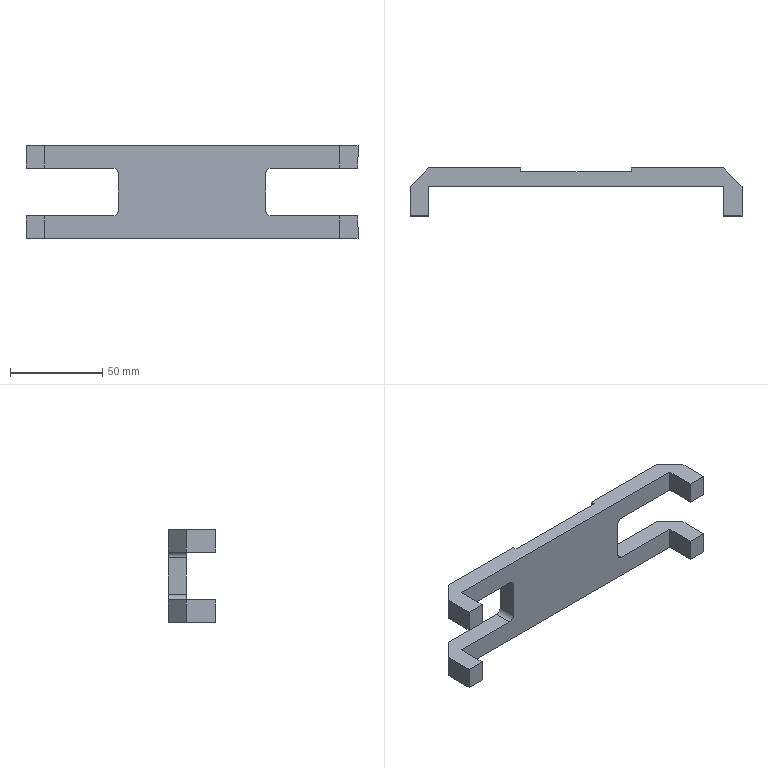Part | SolidWorks | features Cut 2, Chamfer 1, Extrusion 1, Fillet 1, ICE 1, MirrorPattern 1 | 1 solid | 34 faces | box 180 x 26 x 50 mm | volume 63357 mm3 | plane 30 | cylinder 4 | commonest cylinder face diameters 6 x4
STEP:
#1=CARTESIAN_POINT('',(30.,10.,25.));
#2=VERTEX_POINT('',#1);
#3=CARTESIAN_POINT('',(30.,10.,-25.));
#4=VERTEX_POINT('',#3);
#5=CARTESIAN_POINT('',(30.,10.,25.));
#6=DIRECTION('',(0.,0.,-1.));
#7=VECTOR('',#6,1000.);
#8=LINE('',#5,#7);
#9=EDGE_CURVE('',#2,#4,#8,.T.);
#10=ORIENTED_EDGE('',*,*,#9,.F.);
#11=CARTESIAN_POINT('',(80.,10.,25.));
#12=VERTEX_POINT('',#11);
#13=CARTESIAN_POINT('',(-90.,10.,25.));
#14=DIRECTION('',(1.,0.,0.));
#15=VECTOR('',#14,1000.);
#16=LINE('',#13,#15);
#17=EDGE_CURVE('',#2,#12,#16,.T.);
#18=ORIENTED_EDGE('',*,*,#17,.T.);
#19=CARTESIAN_POINT('',(80.,10.,13.));
#20=VERTEX_POINT('',#19);
#21=CARTESIAN_POINT('',(80.,10.,13.));
#22=DIRECTION('',(0.,0.,-1.));
#23=VECTOR('',#22,1000.);
#24=LINE('',#21,#23);
#25=EDGE_CURVE('',#12,#20,#24,.T.);
#26=ORIENTED_EDGE('',*,*,#25,.T.);
#27=CARTESIAN_POINT('',(43.,10.,13.));
#28=VERTEX_POINT('',#27);
#29=CARTESIAN_POINT('',(90.,10.,13.));
#30=DIRECTION('',(-1.,0.,0.));
#31=VECTOR('',#30,1000.);
#32=LINE('',#29,#31);
#33=EDGE_CURVE('',#20,#28,#32,.T.);
#34=ORIENTED_EDGE('',*,*,#33,.T.);
#35=CARTESIAN_POINT('',(40.,10.,10.));
#36=VERTEX_POINT('',#35);
#37=CARTESIAN_POINT('',(43.,10.,10.));
#38=DIRECTION('',(0.,-1.,0.));
#39=DIRECTION('',(0.,0.,1.));
#40=AXIS2_PLACEMENT_3D('',#37,#38,#39);
#41=CIRCLE('',#40,3.);
#42=EDGE_CURVE('',#28,#36,#41,.T.);
#43=ORIENTED_EDGE('',*,*,#42,.T.);
#44=CARTESIAN_POINT('',(40.,10.,-10.));
#45=VERTEX_POINT('',#44);
#46=CARTESIAN_POINT('',(40.,10.,-13.));
#47=DIRECTION('',(0.,0.,-1.));
#48=VECTOR('',#47,1000.);
#49=LINE('',#46,#48);
#50=EDGE_CURVE('',#36,#45,#49,.T.);
#51=ORIENTED_EDGE('',*,*,#50,.T.);
#52=CARTESIAN_POINT('',(43.,10.,-13.));
#53=VERTEX_POINT('',#52);
#54=CARTESIAN_POINT('',(43.,10.,-10.));
#55=DIRECTION('',(0.,-1.,0.));
#56=DIRECTION('',(0.,0.,1.));
#57=AXIS2_PLACEMENT_3D('',#54,#55,#56);
#58=CIRCLE('',#57,3.);
#59=EDGE_CURVE('',#45,#53,#58,.T.);
#60=ORIENTED_EDGE('',*,*,#59,.T.);
#61=CARTESIAN_POINT('',(80.,10.,-13.));
#62=VERTEX_POINT('',#61);
#63=CARTESIAN_POINT('',(90.,10.,-13.));
#64=DIRECTION('',(1.,0.,0.));
#65=VECTOR('',#64,1000.);
#66=LINE('',#63,#65);
#67=EDGE_CURVE('',#53,#62,#66,.T.);
#68=ORIENTED_EDGE('',*,*,#67,.T.);
#69=CARTESIAN_POINT('',(80.,10.,-25.));
#70=VERTEX_POINT('',#69);
#71=CARTESIAN_POINT('',(80.,10.,-25.));
#72=DIRECTION('',(0.,0.,-1.));
#73=VECTOR('',#72,1000.);
#74=LINE('',#71,#73);
#75=EDGE_CURVE('',#62,#70,#74,.T.);
#76=ORIENTED_EDGE('',*,*,#75,.T.);
#77=CARTESIAN_POINT('',(-90.,10.,-25.));
#78=DIRECTION('',(-1.,0.,0.));
#79=VECTOR('',#78,1000.);
#80=LINE('',#77,#79);
#81=EDGE_CURVE('',#70,#4,#80,.T.);
#82=ORIENTED_EDGE('',*,*,#81,.T.);
#83=EDGE_LOOP('',(#10,#18,#26,#34,#43,#51,#60,#68,#76,#82));
#84=FACE_OUTER_BOUND('',#83,.T.);
#85=CARTESIAN_POINT('',(0.,10.,0.));
#86=DIRECTION('',(0.,1.,0.));
#87=DIRECTION('',(0.,0.,1.));
#88=AXIS2_PLACEMENT_3D('',#85,#86,#87);
#89=PLANE('',#88);
#90=ADVANCED_FACE('',(#84),#89,.T.);
#91=CARTESIAN_POINT('',(80.,0.,13.));
#92=VERTEX_POINT('',#91);
#93=CARTESIAN_POINT('',(43.,0.,13.));
#94=VERTEX_POINT('',#93);
#95=CARTESIAN_POINT('',(0.,0.,13.));
#96=DIRECTION('',(-1.,0.,0.));
#97=VECTOR('',#96,1000.);
#98=LINE('',#95,#97);
#99=EDGE_CURVE('',#92,#94,#98,.T.);
#100=ORIENTED_EDGE('',*,*,#99,.F.);
#101=CARTESIAN_POINT('',(80.,0.,25.));
#102=VERTEX_POINT('',#101);
#103=CARTESIAN_POINT('',(80.,0.,-25.));
#104=DIRECTION('',(0.,0.,-1.));
#105=VECTOR('',#104,1000.);
#106=LINE('',#103,#105);
#107=EDGE_CURVE('',#102,#92,#106,.T.);
#108=ORIENTED_EDGE('',*,*,#107,.F.);
#109=CARTESIAN_POINT('',(-80.,0.,25.));
#110=VERTEX_POINT('',#109);
#111=CARTESIAN_POINT('',(-90.,0.,25.));
#112=DIRECTION('',(1.,0.,0.));
#113=VECTOR('',#112,1000.);
#114=LINE('',#111,#113);
#115=EDGE_CURVE('',#110,#102,#114,.T.);
#116=ORIENTED_EDGE('',*,*,#115,.F.);
#117=CARTESIAN_POINT('',(-80.,0.,13.));
#118=VERTEX_POINT('',#117);
#119=CARTESIAN_POINT('',(-80.,0.,-25.));
#120=DIRECTION('',(0.,0.,1.));
#121=VECTOR('',#120,1000.);
#122=LINE('',#119,#121);
#123=EDGE_CURVE('',#118,#110,#122,.T.);
#124=ORIENTED_EDGE('',*,*,#123,.F.);
#125=CARTESIAN_POINT('',(-43.,0.,13.));
#126=VERTEX_POINT('',#125);
#127=CARTESIAN_POINT('',(0.,0.,13.));
#128=DIRECTION('',(1.,0.,0.));
#129=VECTOR('',#128,1000.);
#130=LINE('',#127,#129);
#131=EDGE_CURVE('',#118,#126,#130,.T.);
#132=ORIENTED_EDGE('',*,*,#131,.T.);
#133=CARTESIAN_POINT('',(-40.,0.,10.));
#134=VERTEX_POINT('',#133);
#135=CARTESIAN_POINT('',(-43.,0.,10.));
#136=DIRECTION('',(0.,1.,0.));
#137=DIRECTION('',(0.,0.,1.));
#138=AXIS2_PLACEMENT_3D('',#135,#136,#137);
#139=CIRCLE('',#138,3.);
#140=EDGE_CURVE('',#126,#134,#139,.T.);
#141=ORIENTED_EDGE('',*,*,#140,.T.);
#142=CARTESIAN_POINT('',(-40.,0.,-10.));
#143=VERTEX_POINT('',#142);
#144=CARTESIAN_POINT('',(-40.,0.,0.));
#145=DIRECTION('',(0.,0.,-1.));
#146=VECTOR('',#145,1000.);
#147=LINE('',#144,#146);
#148=EDGE_CURVE('',#134,#143,#147,.T.);
#149=ORIENTED_EDGE('',*,*,#148,.T.);
#150=CARTESIAN_POINT('',(-43.,0.,-13.));
#151=VERTEX_POINT('',#150);
#152=CARTESIAN_POINT('',(-43.,0.,-10.));
#153=DIRECTION('',(0.,1.,0.));
#154=DIRECTION('',(0.,0.,1.));
#155=AXIS2_PLACEMENT_3D('',#152,#153,#154);
#156=CIRCLE('',#155,3.);
#157=EDGE_CURVE('',#143,#151,#156,.T.);
#158=ORIENTED_EDGE('',*,*,#157,.T.);
#159=CARTESIAN_POINT('',(-80.,0.,-13.));
#160=VERTEX_POINT('',#159);
#161=CARTESIAN_POINT('',(0.,0.,-13.));
#162=DIRECTION('',(-1.,0.,0.));
#163=VECTOR('',#162,1000.);
#164=LINE('',#161,#163);
#165=EDGE_CURVE('',#151,#160,#164,.T.);
#166=ORIENTED_EDGE('',*,*,#165,.T.);
#167=CARTESIAN_POINT('',(-80.,0.,-25.));
#168=VERTEX_POINT('',#167);
#169=CARTESIAN_POINT('',(-80.,0.,-25.));
#170=DIRECTION('',(0.,0.,1.));
#171=VECTOR('',#170,1000.);
#172=LINE('',#169,#171);
#173=EDGE_CURVE('',#168,#160,#172,.T.);
#174=ORIENTED_EDGE('',*,*,#173,.F.);
#175=CARTESIAN_POINT('',(80.,0.,-25.));
#176=VERTEX_POINT('',#175);
#177=CARTESIAN_POINT('',(-90.,0.,-25.));
#178=DIRECTION('',(-1.,0.,0.));
#179=VECTOR('',#178,1000.);
#180=LINE('',#177,#179);
#181=EDGE_CURVE('',#176,#168,#180,.T.);
#182=ORIENTED_EDGE('',*,*,#181,.F.);
#183=CARTESIAN_POINT('',(80.,0.,-13.));
#184=VERTEX_POINT('',#183);
#185=CARTESIAN_POINT('',(80.,0.,-25.));
#186=DIRECTION('',(0.,0.,-1.));
#187=VECTOR('',#186,1000.);
#188=LINE('',#185,#187);
#189=EDGE_CURVE('',#184,#176,#188,.T.);
#190=ORIENTED_EDGE('',*,*,#189,.F.);
#191=CARTESIAN_POINT('',(43.,0.,-13.));
#192=VERTEX_POINT('',#191);
#193=CARTESIAN_POINT('',(0.,0.,-13.));
#194=DIRECTION('',(1.,0.,0.));
#195=VECTOR('',#194,1000.);
#196=LINE('',#193,#195);
#197=EDGE_CURVE('',#192,#184,#196,.T.);
#198=ORIENTED_EDGE('',*,*,#197,.F.);
#199=CARTESIAN_POINT('',(40.,0.,-10.));
#200=VERTEX_POINT('',#199);
#201=CARTESIAN_POINT('',(43.,0.,-10.));
#202=DIRECTION('',(0.,1.,0.));
#203=DIRECTION('',(0.,0.,1.));
#204=AXIS2_PLACEMENT_3D('',#201,#202,#203);
#205=CIRCLE('',#204,3.);
#206=EDGE_CURVE('',#192,#200,#205,.T.);
#207=ORIENTED_EDGE('',*,*,#206,.T.);
#208=CARTESIAN_POINT('',(40.,0.,10.));
#209=VERTEX_POINT('',#208);
#210=CARTESIAN_POINT('',(40.,0.,0.));
#211=DIRECTION('',(0.,0.,-1.));
#212=VECTOR('',#211,1000.);
#213=LINE('',#210,#212);
#214=EDGE_CURVE('',#209,#200,#213,.T.);
#215=ORIENTED_EDGE('',*,*,#214,.F.);
#216=CARTESIAN_POINT('',(43.,0.,10.));
#217=DIRECTION('',(0.,1.,0.));
#218=DIRECTION('',(0.,0.,1.));
#219=AXIS2_PLACEMENT_3D('',#216,#217,#218);
#220=CIRCLE('',#219,3.);
#221=EDGE_CURVE('',#209,#94,#220,.T.);
#222=ORIENTED_EDGE('',*,*,#221,.T.);
#223=EDGE_LOOP('',(#100,#108,#116,#124,#132,#141,#149,#158,#166,#174,#182,#190,#198,#207,#215,#222));
#224=FACE_OUTER_BOUND('',#223,.T.);
#225=CARTESIAN_POINT('',(0.,0.,0.));
#226=DIRECTION('',(0.,1.,0.));
#227=DIRECTION('',(0.,0.,1.));
#228=AXIS2_PLACEMENT_3D('',#225,#226,#227);
#229=PLANE('',#228);
#230=ADVANCED_FACE('',(#224),#229,.F.);
#231=CARTESIAN_POINT('',(90.,-16.,13.));
#232=VERTEX_POINT('',#231);
#233=CARTESIAN_POINT('',(90.,0.,13.));
#234=VERTEX_POINT('',#233);
#235=CARTESIAN_POINT('',(90.,-16.,13.));
#236=DIRECTION('',(0.,1.,0.));
#237=VECTOR('',#236,1000.);
#238=LINE('',#235,#237);
#239=EDGE_CURVE('',#232,#234,#238,.T.);
#240=ORIENTED_EDGE('',*,*,#239,.T.);
#241=CARTESIAN_POINT('',(90.,0.,25.));
#242=VERTEX_POINT('',#241);
#243=CARTESIAN_POINT('',(90.,0.,25.));
#244=DIRECTION('',(0.,0.,1.));
#245=VECTOR('',#244,1000.);
#246=LINE('',#243,#245);
#247=EDGE_CURVE('',#234,#242,#246,.T.);
#248=ORIENTED_EDGE('',*,*,#247,.T.);
#249=CARTESIAN_POINT('',(90.,-16.,25.));
#250=VERTEX_POINT('',#249);
#251=CARTESIAN_POINT('',(90.,10.,25.));
#252=DIRECTION('',(0.,-1.,0.));
#253=VECTOR('',#252,1000.);
#254=LINE('',#251,#253);
#255=EDGE_CURVE('',#242,#250,#254,.T.);
#256=ORIENTED_EDGE('',*,*,#255,.T.);
#257=CARTESIAN_POINT('',(90.,-16.,-25.));
#258=DIRECTION('',(0.,0.,1.));
#259=VECTOR('',#258,1000.);
#260=LINE('',#257,#259);
#261=EDGE_CURVE('',#232,#250,#260,.T.);
#262=ORIENTED_EDGE('',*,*,#261,.F.);
#263=EDGE_LOOP('',(#240,#248,#256,#262));
#264=FACE_OUTER_BOUND('',#263,.T.);
#265=CARTESIAN_POINT('',(90.,10.,-25.));
#266=DIRECTION('',(-1.,0.,0.));
#267=DIRECTION('',(0.,0.,1.));
#268=AXIS2_PLACEMENT_3D('',#265,#266,#267);
#269=PLANE('',#268);
#270=ADVANCED_FACE('',(#264),#269,.F.);
#271=CARTESIAN_POINT('',(90.,0.,-25.));
#272=VERTEX_POINT('',#271);
#273=CARTESIAN_POINT('',(90.,-16.,-25.));
#274=VERTEX_POINT('',#273);
#275=CARTESIAN_POINT('',(90.,10.,-25.));
#276=DIRECTION('',(0.,-1.,0.));
#277=VECTOR('',#276,1000.);
#278=LINE('',#275,#277);
#279=EDGE_CURVE('',#272,#274,#278,.T.);
#280=ORIENTED_EDGE('',*,*,#279,.F.);
#281=CARTESIAN_POINT('',(90.,0.,-13.));
#282=VERTEX_POINT('',#281);
#283=CARTESIAN_POINT('',(90.,0.,-13.));
#284=DIRECTION('',(0.,0.,1.));
#285=VECTOR('',#284,1000.);
#286=LINE('',#283,#285);
#287=EDGE_CURVE('',#272,#282,#286,.T.);
#288=ORIENTED_EDGE('',*,*,#287,.T.);
#289=CARTESIAN_POINT('',(90.,-16.,-13.));
#290=VERTEX_POINT('',#289);
#291=CARTESIAN_POINT('',(90.,-16.,-13.));
#292=DIRECTION('',(0.,1.,0.));
#293=VECTOR('',#292,1000.);
#294=LINE('',#291,#293);
#295=EDGE_CURVE('',#290,#282,#294,.T.);
#296=ORIENTED_EDGE('',*,*,#295,.F.);
#297=CARTESIAN_POINT('',(90.,-16.,-25.));
#298=DIRECTION('',(0.,0.,1.));
#299=VECTOR('',#298,1000.);
#300=LINE('',#297,#299);
#301=EDGE_CURVE('',#274,#290,#300,.T.);
#302=ORIENTED_EDGE('',*,*,#301,.F.);
#303=EDGE_LOOP('',(#280,#288,#296,#302));
#304=FACE_OUTER_BOUND('',#303,.T.);
#305=CARTESIAN_POINT('',(90.,10.,-25.));
#306=DIRECTION('',(-1.,0.,0.));
#307=DIRECTION('',(0.,0.,1.));
#308=AXIS2_PLACEMENT_3D('',#305,#306,#307);
#309=PLANE('',#308);
#310=ADVANCED_FACE('',(#304),#309,.F.);
#311=CARTESIAN_POINT('',(-30.,10.,-25.));
#312=VERTEX_POINT('',#311);
#313=CARTESIAN_POINT('',(-30.,10.,25.));
#314=VERTEX_POINT('',#313);
#315=CARTESIAN_POINT('',(-30.,10.,25.));
#316=DIRECTION('',(0.,0.,1.));
#317=VECTOR('',#316,1000.);
#318=LINE('',#315,#317);
#319=EDGE_CURVE('',#312,#314,#318,.T.);
#320=ORIENTED_EDGE('',*,*,#319,.F.);
#321=CARTESIAN_POINT('',(-80.,10.,-25.));
#322=VERTEX_POINT('',#321);
#323=CARTESIAN_POINT('',(-90.,10.,-25.));
#324=DIRECTION('',(-1.,0.,0.));
#325=VECTOR('',#324,1000.);
#326=LINE('',#323,#325);
#327=EDGE_CURVE('',#312,#322,#326,.T.);
#328=ORIENTED_EDGE('',*,*,#327,.T.);
#329=CARTESIAN_POINT('',(-80.,10.,-13.));
#330=VERTEX_POINT('',#329);
#331=CARTESIAN_POINT('',(-80.,10.,-13.));
#332=DIRECTION('',(0.,0.,1.));
#333=VECTOR('',#332,1000.);
#334=LINE('',#331,#333);
#335=EDGE_CURVE('',#322,#330,#334,.T.);
#336=ORIENTED_EDGE('',*,*,#335,.T.);
#337=CARTESIAN_POINT('',(-43.,10.,-13.));
#338=VERTEX_POINT('',#337);
#339=CARTESIAN_POINT('',(-90.,10.,-13.));
#340=DIRECTION('',(-1.,0.,0.));
#341=VECTOR('',#340,1000.);
#342=LINE('',#339,#341);
#343=EDGE_CURVE('',#338,#330,#342,.T.);
#344=ORIENTED_EDGE('',*,*,#343,.F.);
#345=CARTESIAN_POINT('',(-40.,10.,-10.));
#346=VERTEX_POINT('',#345);
#347=CARTESIAN_POINT('',(-43.,10.,-10.));
#348=DIRECTION('',(0.,-1.,0.));
#349=DIRECTION('',(0.,0.,1.));
#350=AXIS2_PLACEMENT_3D('',#347,#348,#349);
#351=CIRCLE('',#350,3.);
#352=EDGE_CURVE('',#338,#346,#351,.T.);
#353=ORIENTED_EDGE('',*,*,#352,.T.);
#354=CARTESIAN_POINT('',(-40.,10.,10.));
#355=VERTEX_POINT('',#354);
#356=CARTESIAN_POINT('',(-40.,10.,-13.));
#357=DIRECTION('',(0.,0.,-1.));
#358=VECTOR('',#357,1000.);
#359=LINE('',#356,#358);
#360=EDGE_CURVE('',#355,#346,#359,.T.);
#361=ORIENTED_EDGE('',*,*,#360,.F.);
#362=CARTESIAN_POINT('',(-43.,10.,13.));
#363=VERTEX_POINT('',#362);
#364=CARTESIAN_POINT('',(-43.,10.,10.));
#365=DIRECTION('',(0.,-1.,0.));
#366=DIRECTION('',(0.,0.,1.));
#367=AXIS2_PLACEMENT_3D('',#364,#365,#366);
#368=CIRCLE('',#367,3.);
#369=EDGE_CURVE('',#355,#363,#368,.T.);
#370=ORIENTED_EDGE('',*,*,#369,.T.);
#371=CARTESIAN_POINT('',(-80.,10.,13.));
#372=VERTEX_POINT('',#371);
#373=CARTESIAN_POINT('',(-90.,10.,13.));
#374=DIRECTION('',(1.,0.,0.));
#375=VECTOR('',#374,1000.);
#376=LINE('',#373,#375);
#377=EDGE_CURVE('',#372,#363,#376,.T.);
#378=ORIENTED_EDGE('',*,*,#377,.F.);
#379=CARTESIAN_POINT('',(-80.,10.,25.));
#380=VERTEX_POINT('',#379);
#381=CARTESIAN_POINT('',(-80.,10.,25.));
#382=DIRECTION('',(0.,0.,1.));
#383=VECTOR('',#382,1000.);
#384=LINE('',#381,#383);
#385=EDGE_CURVE('',#372,#380,#384,.T.);
#386=ORIENTED_EDGE('',*,*,#385,.T.);
#387=CARTESIAN_POINT('',(-90.,10.,25.));
#388=DIRECTION('',(1.,0.,0.));
#389=VECTOR('',#388,1000.);
#390=LINE('',#387,#389);
#391=EDGE_CURVE('',#380,#314,#390,.T.);
#392=ORIENTED_EDGE('',*,*,#391,.T.);
#393=EDGE_LOOP('',(#320,#328,#336,#344,#353,#361,#370,#378,#386,#392));
#394=FACE_OUTER_BOUND('',#393,.T.);
#395=CARTESIAN_POINT('',(0.,10.,0.));
#396=DIRECTION('',(0.,1.,0.));
#397=DIRECTION('',(0.,0.,1.));
#398=AXIS2_PLACEMENT_3D('',#395,#396,#397);
#399=PLANE('',#398);
#400=ADVANCED_FACE('',(#394),#399,.T.);
#401=CARTESIAN_POINT('',(80.,-16.,13.));
#402=VERTEX_POINT('',#401);
#403=CARTESIAN_POINT('',(80.,-16.,13.));
#404=DIRECTION('',(0.,1.,0.));
#405=VECTOR('',#404,1000.);
#406=LINE('',#403,#405);
#407=EDGE_CURVE('',#402,#92,#406,.T.);
#408=ORIENTED_EDGE('',*,*,#407,.F.);
#409=CARTESIAN_POINT('',(80.,-16.,25.));
#410=VERTEX_POINT('',#409);
#411=CARTESIAN_POINT('',(80.,-16.,-25.));
#412=DIRECTION('',(0.,0.,-1.));
#413=VECTOR('',#412,1000.);
#414=LINE('',#411,#413);
#415=EDGE_CURVE('',#410,#402,#414,.T.);
#416=ORIENTED_EDGE('',*,*,#415,.F.);
#417=CARTESIAN_POINT('',(80.,-16.,25.));
#418=DIRECTION('',(0.,1.,0.));
#419=VECTOR('',#418,1000.);
#420=LINE('',#417,#419);
#421=EDGE_CURVE('',#410,#102,#420,.T.);
#422=ORIENTED_EDGE('',*,*,#421,.T.);
#423=ORIENTED_EDGE('',*,*,#107,.T.);
#424=EDGE_LOOP('',(#408,#416,#422,#423));
#425=FACE_OUTER_BOUND('',#424,.T.);
#426=CARTESIAN_POINT('',(80.,-16.,-25.));
#427=DIRECTION('',(1.,0.,0.));
#428=DIRECTION('',(0.,0.,-1.));
#429=AXIS2_PLACEMENT_3D('',#426,#427,#428);
#430=PLANE('',#429);
#431=ADVANCED_FACE('',(#425),#430,.F.);
#432=CARTESIAN_POINT('',(80.,-16.,-13.));
#433=VERTEX_POINT('',#432);
#434=CARTESIAN_POINT('',(80.,-16.,-13.));
#435=DIRECTION('',(0.,-1.,0.));
#436=VECTOR('',#435,1000.);
#437=LINE('',#434,#436);
#438=EDGE_CURVE('',#184,#433,#437,.T.);
#439=ORIENTED_EDGE('',*,*,#438,.F.);
#440=ORIENTED_EDGE('',*,*,#189,.T.);
#441=CARTESIAN_POINT('',(80.,-16.,-25.));
#442=VERTEX_POINT('',#441);
#443=CARTESIAN_POINT('',(80.,-16.,-25.));
#444=DIRECTION('',(0.,1.,0.));
#445=VECTOR('',#444,1000.);
#446=LINE('',#443,#445);
#447=EDGE_CURVE('',#442,#176,#446,.T.);
#448=ORIENTED_EDGE('',*,*,#447,.F.);
#449=CARTESIAN_POINT('',(80.,-16.,-25.));
#450=DIRECTION('',(0.,0.,-1.));
#451=VECTOR('',#450,1000.);
#452=LINE('',#449,#451);
#453=EDGE_CURVE('',#433,#442,#452,.T.);
#454=ORIENTED_EDGE('',*,*,#453,.F.);
#455=EDGE_LOOP('',(#439,#440,#448,#454));
#456=FACE_OUTER_BOUND('',#455,.T.);
#457=CARTESIAN_POINT('',(80.,-16.,-25.));
#458=DIRECTION('',(1.,0.,0.));
#459=DIRECTION('',(0.,0.,-1.));
#460=AXIS2_PLACEMENT_3D('',#457,#458,#459);
#461=PLANE('',#460);
#462=ADVANCED_FACE('',(#456),#461,.F.);
#463=ORIENTED_EDGE('',*,*,#415,.T.);
#464=CARTESIAN_POINT('',(0.,-16.,13.));
#465=DIRECTION('',(1.,0.,0.));
#466=VECTOR('',#465,1000.);
#467=LINE('',#464,#466);
#468=EDGE_CURVE('',#402,#232,#467,.T.);
#469=ORIENTED_EDGE('',*,*,#468,.T.);
#470=ORIENTED_EDGE('',*,*,#261,.T.);
#471=CARTESIAN_POINT('',(90.,-16.,25.));
#472=DIRECTION('',(-1.,0.,0.));
#473=VECTOR('',#472,1000.);
#474=LINE('',#471,#473);
#475=EDGE_CURVE('',#250,#410,#474,.T.);
#476=ORIENTED_EDGE('',*,*,#475,.T.);
#477=EDGE_LOOP('',(#463,#469,#470,#476));
#478=FACE_OUTER_BOUND('',#477,.T.);
#479=CARTESIAN_POINT('',(0.,-16.,0.));
#480=DIRECTION('',(0.,-1.,0.));
#481=DIRECTION('',(0.,0.,-1.));
#482=AXIS2_PLACEMENT_3D('',#479,#480,#481);
#483=PLANE('',#482);
#484=ADVANCED_FACE('',(#478),#483,.T.);
#485=ORIENTED_EDGE('',*,*,#301,.T.);
#486=CARTESIAN_POINT('',(0.,-16.,-13.));
#487=DIRECTION('',(-1.,0.,0.));
#488=VECTOR('',#487,1000.);
#489=LINE('',#486,#488);
#490=EDGE_CURVE('',#290,#433,#489,.T.);
#491=ORIENTED_EDGE('',*,*,#490,.T.);
#492=ORIENTED_EDGE('',*,*,#453,.T.);
#493=CARTESIAN_POINT('',(90.,-16.,-25.));
#494=DIRECTION('',(1.,0.,0.));
#495=VECTOR('',#494,1000.);
#496=LINE('',#493,#495);
#497=EDGE_CURVE('',#442,#274,#496,.T.);
#498=ORIENTED_EDGE('',*,*,#497,.T.);
#499=EDGE_LOOP('',(#485,#491,#492,#498));
#500=FACE_OUTER_BOUND('',#499,.T.);
#501=CARTESIAN_POINT('',(0.,-16.,0.));
#502=DIRECTION('',(0.,-1.,0.));
#503=DIRECTION('',(0.,0.,-1.));
#504=AXIS2_PLACEMENT_3D('',#501,#502,#503);
#505=PLANE('',#504);
#506=ADVANCED_FACE('',(#500),#505,.T.);
#507=CARTESIAN_POINT('',(-90.,-16.,-13.));
#508=VERTEX_POINT('',#507);
#509=CARTESIAN_POINT('',(-90.,0.,-13.));
#510=VERTEX_POINT('',#509);
#511=CARTESIAN_POINT('',(-90.,-16.,-13.));
#512=DIRECTION('',(0.,1.,0.));
#513=VECTOR('',#512,1000.);
#514=LINE('',#511,#513);
#515=EDGE_CURVE('',#508,#510,#514,.T.);
#516=ORIENTED_EDGE('',*,*,#515,.T.);
#517=CARTESIAN_POINT('',(-90.,0.,-25.));
#518=VERTEX_POINT('',#517);
#519=CARTESIAN_POINT('',(-90.,0.,-25.));
#520=DIRECTION('',(0.,0.,-1.));
#521=VECTOR('',#520,1000.);
#522=LINE('',#519,#521);
#523=EDGE_CURVE('',#510,#518,#522,.T.);
#524=ORIENTED_EDGE('',*,*,#523,.T.);
#525=CARTESIAN_POINT('',(-90.,-16.,-25.));
#526=VERTEX_POINT('',#525);
#527=CARTESIAN_POINT('',(-90.,10.,-25.));
#528=DIRECTION('',(0.,-1.,0.));
#529=VECTOR('',#528,1000.);
#530=LINE('',#527,#529);
#531=EDGE_CURVE('',#518,#526,#530,.T.);
#532=ORIENTED_EDGE('',*,*,#531,.T.);
#533=CARTESIAN_POINT('',(-90.,-16.,-25.));
#534=DIRECTION('',(0.,0.,-1.));
#535=VECTOR('',#534,1000.);
#536=LINE('',#533,#535);
#537=EDGE_CURVE('',#508,#526,#536,.T.);
#538=ORIENTED_EDGE('',*,*,#537,.F.);
#539=EDGE_LOOP('',(#516,#524,#532,#538));
#540=FACE_OUTER_BOUND('',#539,.T.);
#541=CARTESIAN_POINT('',(-90.,10.,-25.));
#542=DIRECTION('',(1.,0.,0.));
#543=DIRECTION('',(0.,0.,-1.));
#544=AXIS2_PLACEMENT_3D('',#541,#542,#543);
#545=PLANE('',#544);
#546=ADVANCED_FACE('',(#540),#545,.F.);
#547=ORIENTED_EDGE('',*,*,#173,.T.);
#548=CARTESIAN_POINT('',(-80.,-16.,-13.));
#549=VERTEX_POINT('',#548);
#550=CARTESIAN_POINT('',(-80.,-16.,-13.));
#551=DIRECTION('',(0.,-1.,0.));
#552=VECTOR('',#551,1000.);
#553=LINE('',#550,#552);
#554=EDGE_CURVE('',#160,#549,#553,.T.);
#555=ORIENTED_EDGE('',*,*,#554,.T.);
#556=CARTESIAN_POINT('',(-80.,-16.,-25.));
#557=VERTEX_POINT('',#556);
#558=CARTESIAN_POINT('',(-80.,-16.,-25.));
#559=DIRECTION('',(0.,0.,1.));
#560=VECTOR('',#559,1000.);
#561=LINE('',#558,#560);
#562=EDGE_CURVE('',#557,#549,#561,.T.);
#563=ORIENTED_EDGE('',*,*,#562,.F.);
#564=CARTESIAN_POINT('',(-80.,-16.,-25.));
#565=DIRECTION('',(0.,1.,0.));
#566=VECTOR('',#565,1000.);
#567=LINE('',#564,#566);
#568=EDGE_CURVE('',#557,#168,#567,.T.);
#569=ORIENTED_EDGE('',*,*,#568,.T.);
#570=EDGE_LOOP('',(#547,#555,#563,#569));
#571=FACE_OUTER_BOUND('',#570,.T.);
#572=CARTESIAN_POINT('',(-80.,-16.,-25.));
#573=DIRECTION('',(-1.,0.,0.));
#574=DIRECTION('',(0.,0.,1.));
#575=AXIS2_PLACEMENT_3D('',#572,#573,#574);
#576=PLANE('',#575);
#577=ADVANCED_FACE('',(#571),#576,.F.);
#578=ORIENTED_EDGE('',*,*,#562,.T.);
#579=CARTESIAN_POINT('',(0.,-16.,-13.));
#580=DIRECTION('',(-1.,0.,0.));
#581=VECTOR('',#580,1000.);
#582=LINE('',#579,#581);
#583=EDGE_CURVE('',#549,#508,#582,.T.);
#584=ORIENTED_EDGE('',*,*,#583,.T.);
#585=ORIENTED_EDGE('',*,*,#537,.T.);
#586=CARTESIAN_POINT('',(-90.,-16.,-25.));
#587=DIRECTION('',(1.,0.,0.));
#588=VECTOR('',#587,1000.);
#589=LINE('',#586,#588);
#590=EDGE_CURVE('',#526,#557,#589,.T.);
#591=ORIENTED_EDGE('',*,*,#590,.T.);
#592=EDGE_LOOP('',(#578,#584,#585,#591));
#593=FACE_OUTER_BOUND('',#592,.T.);
#594=CARTESIAN_POINT('',(0.,-16.,0.));
#595=DIRECTION('',(0.,1.,0.));
#596=DIRECTION('',(0.,0.,1.));
#597=AXIS2_PLACEMENT_3D('',#594,#595,#596);
#598=PLANE('',#597);
#599=ADVANCED_FACE('',(#593),#598,.F.);
#600=CARTESIAN_POINT('',(30.,8.,-25.));
#601=VERTEX_POINT('',#600);
#602=CARTESIAN_POINT('',(-30.,8.,-25.));
#603=VERTEX_POINT('',#602);
#604=CARTESIAN_POINT('',(30.,8.,-25.));
#605=DIRECTION('',(-1.,0.,0.));
#606=VECTOR('',#605,1000.);
#607=LINE('',#604,#606);
#608=EDGE_CURVE('',#601,#603,#607,.T.);
#609=ORIENTED_EDGE('',*,*,#608,.F.);
#610=CARTESIAN_POINT('',(30.,8.,-25.));
#611=DIRECTION('',(0.,1.,0.));
#612=VECTOR('',#611,1000.);
#613=LINE('',#610,#612);
#614=EDGE_CURVE('',#601,#4,#613,.T.);
#615=ORIENTED_EDGE('',*,*,#614,.T.);
#616=ORIENTED_EDGE('',*,*,#81,.F.);
#617=CARTESIAN_POINT('',(80.,10.,-25.));
#618=DIRECTION('',(0.7071,-0.7071,0.));
#619=VECTOR('',#618,1000.);
#620=LINE('',#617,#619);
#621=EDGE_CURVE('',#70,#272,#620,.T.);
#622=ORIENTED_EDGE('',*,*,#621,.T.);
#623=ORIENTED_EDGE('',*,*,#279,.T.);
#624=ORIENTED_EDGE('',*,*,#497,.F.);
#625=ORIENTED_EDGE('',*,*,#447,.T.);
#626=ORIENTED_EDGE('',*,*,#181,.T.);
#627=ORIENTED_EDGE('',*,*,#568,.F.);
#628=ORIENTED_EDGE('',*,*,#590,.F.);
#629=ORIENTED_EDGE('',*,*,#531,.F.);
#630=CARTESIAN_POINT('',(-80.,10.,-25.));
#631=DIRECTION('',(0.7071,0.7071,0.));
#632=VECTOR('',#631,1000.);
#633=LINE('',#630,#632);
#634=EDGE_CURVE('',#518,#322,#633,.T.);
#635=ORIENTED_EDGE('',*,*,#634,.T.);
#636=ORIENTED_EDGE('',*,*,#327,.F.);
#637=CARTESIAN_POINT('',(-30.,8.,-25.));
#638=DIRECTION('',(0.,1.,0.));
#639=VECTOR('',#638,1000.);
#640=LINE('',#637,#639);
#641=EDGE_CURVE('',#603,#312,#640,.T.);
#642=ORIENTED_EDGE('',*,*,#641,.F.);
#643=EDGE_LOOP('',(#609,#615,#616,#622,#623,#624,#625,#626,#627,#628,#629,#635,#636,#642));
#644=FACE_OUTER_BOUND('',#643,.T.);
#645=CARTESIAN_POINT('',(-90.,10.,-25.));
#646=DIRECTION('',(0.,0.,1.));
#647=DIRECTION('',(1.,0.,0.));
#648=AXIS2_PLACEMENT_3D('',#645,#646,#647);
#649=PLANE('',#648);
#650=ADVANCED_FACE('',(#644),#649,.F.);
#651=CARTESIAN_POINT('',(-90.,0.,25.));
#652=VERTEX_POINT('',#651);
#653=CARTESIAN_POINT('',(-90.,-16.,25.));
#654=VERTEX_POINT('',#653);
#655=CARTESIAN_POINT('',(-90.,10.,25.));
#656=DIRECTION('',(0.,-1.,0.));
#657=VECTOR('',#656,1000.);
#658=LINE('',#655,#657);
#659=EDGE_CURVE('',#652,#654,#658,.T.);
#660=ORIENTED_EDGE('',*,*,#659,.F.);
#661=CARTESIAN_POINT('',(-90.,0.,13.));
#662=VERTEX_POINT('',#661);
#663=CARTESIAN_POINT('',(-90.,0.,13.));
#664=DIRECTION('',(0.,0.,-1.));
#665=VECTOR('',#664,1000.);
#666=LINE('',#663,#665);
#667=EDGE_CURVE('',#652,#662,#666,.T.);
#668=ORIENTED_EDGE('',*,*,#667,.T.);
#669=CARTESIAN_POINT('',(-90.,-16.,13.));
#670=VERTEX_POINT('',#669);
#671=CARTESIAN_POINT('',(-90.,-16.,13.));
#672=DIRECTION('',(0.,1.,0.));
#673=VECTOR('',#672,1000.);
#674=LINE('',#671,#673);
#675=EDGE_CURVE('',#670,#662,#674,.T.);
#676=ORIENTED_EDGE('',*,*,#675,.F.);
#677=CARTESIAN_POINT('',(-90.,-16.,-25.));
#678=DIRECTION('',(0.,0.,-1.));
#679=VECTOR('',#678,1000.);
#680=LINE('',#677,#679);
#681=EDGE_CURVE('',#654,#670,#680,.T.);
#682=ORIENTED_EDGE('',*,*,#681,.F.);
#683=EDGE_LOOP('',(#660,#668,#676,#682));
#684=FACE_OUTER_BOUND('',#683,.T.);
#685=CARTESIAN_POINT('',(-90.,10.,-25.));
#686=DIRECTION('',(1.,0.,0.));
#687=DIRECTION('',(0.,0.,-1.));
#688=AXIS2_PLACEMENT_3D('',#685,#686,#687);
#689=PLANE('',#688);
#690=ADVANCED_FACE('',(#684),#689,.F.);
#691=ORIENTED_EDGE('',*,*,#17,.F.);
#692=CARTESIAN_POINT('',(30.,8.,25.));
#693=VERTEX_POINT('',#692);
#694=CARTESIAN_POINT('',(30.,8.,25.));
#695=DIRECTION('',(0.,1.,0.));
#696=VECTOR('',#695,1000.);
#697=LINE('',#694,#696);
#698=EDGE_CURVE('',#693,#2,#697,.T.);
#699=ORIENTED_EDGE('',*,*,#698,.F.);
#700=CARTESIAN_POINT('',(-30.,8.,25.));
#701=VERTEX_POINT('',#700);
#702=CARTESIAN_POINT('',(30.,8.,25.));
#703=DIRECTION('',(1.,0.,0.));
#704=VECTOR('',#703,1000.);
#705=LINE('',#702,#704);
#706=EDGE_CURVE('',#701,#693,#705,.T.);
#707=ORIENTED_EDGE('',*,*,#706,.F.);
#708=CARTESIAN_POINT('',(-30.,8.,25.));
#709=DIRECTION('',(0.,1.,0.));
#710=VECTOR('',#709,1000.);
#711=LINE('',#708,#710);
#712=EDGE_CURVE('',#701,#314,#711,.T.);
#713=ORIENTED_EDGE('',*,*,#712,.T.);
#714=ORIENTED_EDGE('',*,*,#391,.F.);
#715=CARTESIAN_POINT('',(-80.,10.,25.));
#716=DIRECTION('',(-0.7071,-0.7071,0.));
#717=VECTOR('',#716,1000.);
#718=LINE('',#715,#717);
#719=EDGE_CURVE('',#380,#652,#718,.T.);
#720=ORIENTED_EDGE('',*,*,#719,.T.);
#721=ORIENTED_EDGE('',*,*,#659,.T.);
#722=CARTESIAN_POINT('',(-80.,-16.,25.));
#723=VERTEX_POINT('',#722);
#724=CARTESIAN_POINT('',(-90.,-16.,25.));
#725=DIRECTION('',(-1.,0.,0.));
#726=VECTOR('',#725,1000.);
#727=LINE('',#724,#726);
#728=EDGE_CURVE('',#723,#654,#727,.T.);
#729=ORIENTED_EDGE('',*,*,#728,.F.);
#730=CARTESIAN_POINT('',(-80.,-16.,25.));
#731=DIRECTION('',(0.,1.,0.));
#732=VECTOR('',#731,1000.);
#733=LINE('',#730,#732);
#734=EDGE_CURVE('',#723,#110,#733,.T.);
#735=ORIENTED_EDGE('',*,*,#734,.T.);
#736=ORIENTED_EDGE('',*,*,#115,.T.);
#737=ORIENTED_EDGE('',*,*,#421,.F.);
#738=ORIENTED_EDGE('',*,*,#475,.F.);
#739=ORIENTED_EDGE('',*,*,#255,.F.);
#740=CARTESIAN_POINT('',(80.,10.,25.));
#741=DIRECTION('',(-0.7071,0.7071,0.));
#742=VECTOR('',#741,1000.);
#743=LINE('',#740,#742);
#744=EDGE_CURVE('',#242,#12,#743,.T.);
#745=ORIENTED_EDGE('',*,*,#744,.T.);
#746=EDGE_LOOP('',(#691,#699,#707,#713,#714,#720,#721,#729,#735,#736,#737,#738,#739,#745));
#747=FACE_OUTER_BOUND('',#746,.T.);
#748=CARTESIAN_POINT('',(-90.,10.,25.));
#749=DIRECTION('',(0.,0.,-1.));
#750=DIRECTION('',(-1.,0.,0.));
#751=AXIS2_PLACEMENT_3D('',#748,#749,#750);
#752=PLANE('',#751);
#753=ADVANCED_FACE('',(#747),#752,.F.);
#754=CARTESIAN_POINT('',(-80.,-16.,13.));
#755=VERTEX_POINT('',#754);
#756=CARTESIAN_POINT('',(-80.,-16.,-25.));
#757=DIRECTION('',(0.,0.,1.));
#758=VECTOR('',#757,1000.);
#759=LINE('',#756,#758);
#760=EDGE_CURVE('',#755,#723,#759,.T.);
#761=ORIENTED_EDGE('',*,*,#760,.F.);
#762=CARTESIAN_POINT('',(-80.,-16.,13.));
#763=DIRECTION('',(0.,1.,0.));
#764=VECTOR('',#763,1000.);
#765=LINE('',#762,#764);
#766=EDGE_CURVE('',#755,#118,#765,.T.);
#767=ORIENTED_EDGE('',*,*,#766,.T.);
#768=ORIENTED_EDGE('',*,*,#123,.T.);
#769=ORIENTED_EDGE('',*,*,#734,.F.);
#770=EDGE_LOOP('',(#761,#767,#768,#769));
#771=FACE_OUTER_BOUND('',#770,.T.);
#772=CARTESIAN_POINT('',(-80.,-16.,-25.));
#773=DIRECTION('',(-1.,0.,0.));
#774=DIRECTION('',(0.,0.,1.));
#775=AXIS2_PLACEMENT_3D('',#772,#773,#774);
#776=PLANE('',#775);
#777=ADVANCED_FACE('',(#771),#776,.F.);
#778=ORIENTED_EDGE('',*,*,#681,.T.);
#779=CARTESIAN_POINT('',(0.,-16.,13.));
#780=DIRECTION('',(1.,0.,0.));
#781=VECTOR('',#780,1000.);
#782=LINE('',#779,#781);
#783=EDGE_CURVE('',#670,#755,#782,.T.);
#784=ORIENTED_EDGE('',*,*,#783,.T.);
#785=ORIENTED_EDGE('',*,*,#760,.T.);
#786=ORIENTED_EDGE('',*,*,#728,.T.);
#787=EDGE_LOOP('',(#778,#784,#785,#786));
#788=FACE_OUTER_BOUND('',#787,.T.);
#789=CARTESIAN_POINT('',(0.,-16.,0.));
#790=DIRECTION('',(0.,1.,0.));
#791=DIRECTION('',(0.,0.,1.));
#792=AXIS2_PLACEMENT_3D('',#789,#790,#791);
#793=PLANE('',#792);
#794=ADVANCED_FACE('',(#788),#793,.F.);
#795=ORIENTED_EDGE('',*,*,#148,.F.);
#796=CARTESIAN_POINT('',(-40.,10.,10.));
#797=DIRECTION('',(0.,1.,0.));
#798=VECTOR('',#797,1000.);
#799=LINE('',#796,#798);
#800=EDGE_CURVE('',#134,#355,#799,.T.);
#801=ORIENTED_EDGE('',*,*,#800,.T.);
#802=ORIENTED_EDGE('',*,*,#360,.T.);
#803=CARTESIAN_POINT('',(-40.,0.,-10.));
#804=DIRECTION('',(0.,-1.,0.));
#805=VECTOR('',#804,1000.);
#806=LINE('',#803,#805);
#807=EDGE_CURVE('',#346,#143,#806,.T.);
#808=ORIENTED_EDGE('',*,*,#807,.T.);
#809=EDGE_LOOP('',(#795,#801,#802,#808));
#810=FACE_OUTER_BOUND('',#809,.T.);
#811=CARTESIAN_POINT('',(-40.,-16.,-13.));
#812=DIRECTION('',(1.,0.,0.));
#813=DIRECTION('',(0.,0.,-1.));
#814=AXIS2_PLACEMENT_3D('',#811,#812,#813);
#815=PLANE('',#814);
#816=ADVANCED_FACE('',(#810),#815,.F.);
#817=ORIENTED_EDGE('',*,*,#343,.T.);
#818=CARTESIAN_POINT('',(-80.,10.,-13.));
#819=DIRECTION('',(-0.7071,-0.7071,0.));
#820=VECTOR('',#819,1000.);
#821=LINE('',#818,#820);
#822=EDGE_CURVE('',#330,#510,#821,.T.);
#823=ORIENTED_EDGE('',*,*,#822,.T.);
#824=ORIENTED_EDGE('',*,*,#515,.F.);
#825=ORIENTED_EDGE('',*,*,#583,.F.);
#826=ORIENTED_EDGE('',*,*,#554,.F.);
#827=ORIENTED_EDGE('',*,*,#165,.F.);
#828=CARTESIAN_POINT('',(-43.,10.,-13.));
#829=DIRECTION('',(0.,1.,0.));
#830=VECTOR('',#829,1000.);
#831=LINE('',#828,#830);
#832=EDGE_CURVE('',#151,#338,#831,.T.);
#833=ORIENTED_EDGE('',*,*,#832,.T.);
#834=EDGE_LOOP('',(#817,#823,#824,#825,#826,#827,#833));
#835=FACE_OUTER_BOUND('',#834,.T.);
#836=CARTESIAN_POINT('',(-90.,-16.,-13.));
#837=DIRECTION('',(0.,0.,-1.));
#838=DIRECTION('',(-1.,0.,0.));
#839=AXIS2_PLACEMENT_3D('',#836,#837,#838);
#840=PLANE('',#839);
#841=ADVANCED_FACE('',(#835),#840,.F.);
#842=ORIENTED_EDGE('',*,*,#675,.T.);
#843=CARTESIAN_POINT('',(-80.,10.,13.));
#844=DIRECTION('',(0.7071,0.7071,0.));
#845=VECTOR('',#844,1000.);
#846=LINE('',#843,#845);
#847=EDGE_CURVE('',#662,#372,#846,.T.);
#848=ORIENTED_EDGE('',*,*,#847,.T.);
#849=ORIENTED_EDGE('',*,*,#377,.T.);
#850=CARTESIAN_POINT('',(-43.,0.,13.));
#851=DIRECTION('',(0.,-1.,0.));
#852=VECTOR('',#851,1000.);
#853=LINE('',#850,#852);
#854=EDGE_CURVE('',#363,#126,#853,.T.);
#855=ORIENTED_EDGE('',*,*,#854,.T.);
#856=ORIENTED_EDGE('',*,*,#131,.F.);
#857=ORIENTED_EDGE('',*,*,#766,.F.);
#858=ORIENTED_EDGE('',*,*,#783,.F.);
#859=EDGE_LOOP('',(#842,#848,#849,#855,#856,#857,#858));
#860=FACE_OUTER_BOUND('',#859,.T.);
#861=CARTESIAN_POINT('',(-90.,-16.,13.));
#862=DIRECTION('',(0.,0.,1.));
#863=DIRECTION('',(1.,0.,0.));
#864=AXIS2_PLACEMENT_3D('',#861,#862,#863);
#865=PLANE('',#864);
#866=ADVANCED_FACE('',(#860),#865,.F.);
#867=ORIENTED_EDGE('',*,*,#50,.F.);
#868=CARTESIAN_POINT('',(40.,0.,10.));
#869=DIRECTION('',(0.,-1.,0.));
#870=VECTOR('',#869,1000.);
#871=LINE('',#868,#870);
#872=EDGE_CURVE('',#36,#209,#871,.T.);
#873=ORIENTED_EDGE('',*,*,#872,.T.);
#874=ORIENTED_EDGE('',*,*,#214,.T.);
#875=CARTESIAN_POINT('',(40.,10.,-10.));
#876=DIRECTION('',(0.,1.,0.));
#877=VECTOR('',#876,1000.);
#878=LINE('',#875,#877);
#879=EDGE_CURVE('',#200,#45,#878,.T.);
#880=ORIENTED_EDGE('',*,*,#879,.T.);
#881=EDGE_LOOP('',(#867,#873,#874,#880));
#882=FACE_OUTER_BOUND('',#881,.T.);
#883=CARTESIAN_POINT('',(40.,-16.,-13.));
#884=DIRECTION('',(1.,0.,0.));
#885=DIRECTION('',(0.,0.,-1.));
#886=AXIS2_PLACEMENT_3D('',#883,#884,#885);
#887=PLANE('',#886);
#888=ADVANCED_FACE('',(#882),#887,.T.);
#889=ORIENTED_EDGE('',*,*,#33,.F.);
#890=CARTESIAN_POINT('',(98.,-8.,13.));
#891=DIRECTION('',(0.7071,-0.7071,0.));
#892=VECTOR('',#891,1000.);
#893=LINE('',#890,#892);
#894=EDGE_CURVE('',#20,#234,#893,.T.);
#895=ORIENTED_EDGE('',*,*,#894,.T.);
#896=ORIENTED_EDGE('',*,*,#239,.F.);
#897=ORIENTED_EDGE('',*,*,#468,.F.);
#898=ORIENTED_EDGE('',*,*,#407,.T.);
#899=ORIENTED_EDGE('',*,*,#99,.T.);
#900=CARTESIAN_POINT('',(43.,10.,13.));
#901=DIRECTION('',(0.,1.,0.));
#902=VECTOR('',#901,1000.);
#903=LINE('',#900,#902);
#904=EDGE_CURVE('',#94,#28,#903,.T.);
#905=ORIENTED_EDGE('',*,*,#904,.T.);
#906=EDGE_LOOP('',(#889,#895,#896,#897,#898,#899,#905));
#907=FACE_OUTER_BOUND('',#906,.T.);
#908=CARTESIAN_POINT('',(90.,-16.,13.));
#909=DIRECTION('',(0.,0.,-1.));
#910=DIRECTION('',(-1.,0.,0.));
#911=AXIS2_PLACEMENT_3D('',#908,#909,#910);
#912=PLANE('',#911);
#913=ADVANCED_FACE('',(#907),#912,.T.);
#914=ORIENTED_EDGE('',*,*,#295,.T.);
#915=CARTESIAN_POINT('',(98.,-8.,-13.));
#916=DIRECTION('',(-0.7071,0.7071,0.));
#917=VECTOR('',#916,1000.);
#918=LINE('',#915,#917);
#919=EDGE_CURVE('',#282,#62,#918,.T.);
#920=ORIENTED_EDGE('',*,*,#919,.T.);
#921=ORIENTED_EDGE('',*,*,#67,.F.);
#922=CARTESIAN_POINT('',(43.,0.,-13.));
#923=DIRECTION('',(0.,-1.,0.));
#924=VECTOR('',#923,1000.);
#925=LINE('',#922,#924);
#926=EDGE_CURVE('',#53,#192,#925,.T.);
#927=ORIENTED_EDGE('',*,*,#926,.T.);
#928=ORIENTED_EDGE('',*,*,#197,.T.);
#929=ORIENTED_EDGE('',*,*,#438,.T.);
#930=ORIENTED_EDGE('',*,*,#490,.F.);
#931=EDGE_LOOP('',(#914,#920,#921,#927,#928,#929,#930));
#932=FACE_OUTER_BOUND('',#931,.T.);
#933=CARTESIAN_POINT('',(90.,-16.,-13.));
#934=DIRECTION('',(0.,0.,1.));
#935=DIRECTION('',(1.,0.,0.));
#936=AXIS2_PLACEMENT_3D('',#933,#934,#935);
#937=PLANE('',#936);
#938=ADVANCED_FACE('',(#932),#937,.T.);
#939=ORIENTED_EDGE('',*,*,#221,.F.);
#940=ORIENTED_EDGE('',*,*,#872,.F.);
#941=ORIENTED_EDGE('',*,*,#42,.F.);
#942=ORIENTED_EDGE('',*,*,#904,.F.);
#943=EDGE_LOOP('',(#939,#940,#941,#942));
#944=FACE_OUTER_BOUND('',#943,.T.);
#945=CARTESIAN_POINT('',(43.,-16.,10.));
#946=DIRECTION('',(0.,-1.,0.));
#947=DIRECTION('',(0.,0.,-1.));
#948=AXIS2_PLACEMENT_3D('',#945,#946,#947);
#949=CYLINDRICAL_SURFACE('',#948,3.);
#950=ADVANCED_FACE('',(#944),#949,.F.);
#951=ORIENTED_EDGE('',*,*,#206,.F.);
#952=ORIENTED_EDGE('',*,*,#926,.F.);
#953=ORIENTED_EDGE('',*,*,#59,.F.);
#954=ORIENTED_EDGE('',*,*,#879,.F.);
#955=EDGE_LOOP('',(#951,#952,#953,#954));
#956=FACE_OUTER_BOUND('',#955,.T.);
#957=CARTESIAN_POINT('',(43.,-16.,-10.));
#958=DIRECTION('',(0.,-1.,0.));
#959=DIRECTION('',(0.,0.,-1.));
#960=AXIS2_PLACEMENT_3D('',#957,#958,#959);
#961=CYLINDRICAL_SURFACE('',#960,3.);
#962=ADVANCED_FACE('',(#956),#961,.F.);
#963=ORIENTED_EDGE('',*,*,#140,.F.);
#964=ORIENTED_EDGE('',*,*,#854,.F.);
#965=ORIENTED_EDGE('',*,*,#369,.F.);
#966=ORIENTED_EDGE('',*,*,#800,.F.);
#967=EDGE_LOOP('',(#963,#964,#965,#966));
#968=FACE_OUTER_BOUND('',#967,.T.);
#969=CARTESIAN_POINT('',(-43.,-16.,10.));
#970=DIRECTION('',(0.,-1.,0.));
#971=DIRECTION('',(0.,0.,-1.));
#972=AXIS2_PLACEMENT_3D('',#969,#970,#971);
#973=CYLINDRICAL_SURFACE('',#972,3.);
#974=ADVANCED_FACE('',(#968),#973,.F.);
#975=ORIENTED_EDGE('',*,*,#157,.F.);
#976=ORIENTED_EDGE('',*,*,#807,.F.);
#977=ORIENTED_EDGE('',*,*,#352,.F.);
#978=ORIENTED_EDGE('',*,*,#832,.F.);
#979=EDGE_LOOP('',(#975,#976,#977,#978));
#980=FACE_OUTER_BOUND('',#979,.T.);
#981=CARTESIAN_POINT('',(-43.,-16.,-10.));
#982=DIRECTION('',(0.,-1.,0.));
#983=DIRECTION('',(0.,0.,-1.));
#984=AXIS2_PLACEMENT_3D('',#981,#982,#983);
#985=CYLINDRICAL_SURFACE('',#984,3.);
#986=ADVANCED_FACE('',(#980),#985,.F.);
#987=ORIENTED_EDGE('',*,*,#919,.F.);
#988=ORIENTED_EDGE('',*,*,#287,.F.);
#989=ORIENTED_EDGE('',*,*,#621,.F.);
#990=ORIENTED_EDGE('',*,*,#75,.F.);
#991=EDGE_LOOP('',(#987,#988,#989,#990));
#992=FACE_OUTER_BOUND('',#991,.T.);
#993=CARTESIAN_POINT('',(80.,10.,0.));
#994=DIRECTION('',(0.7071,0.7071,0.));
#995=DIRECTION('',(0.,0.,1.));
#996=AXIS2_PLACEMENT_3D('',#993,#994,#995);
#997=PLANE('',#996);
#998=ADVANCED_FACE('',(#992),#997,.T.);
#999=ORIENTED_EDGE('',*,*,#744,.F.);
#1000=ORIENTED_EDGE('',*,*,#247,.F.);
#1001=ORIENTED_EDGE('',*,*,#894,.F.);
#1002=ORIENTED_EDGE('',*,*,#25,.F.);
#1003=EDGE_LOOP('',(#999,#1000,#1001,#1002));
#1004=FACE_OUTER_BOUND('',#1003,.T.);
#1005=CARTESIAN_POINT('',(80.,10.,0.));
#1006=DIRECTION('',(0.7071,0.7071,0.));
#1007=DIRECTION('',(0.,0.,1.));
#1008=AXIS2_PLACEMENT_3D('',#1005,#1006,#1007);
#1009=PLANE('',#1008);
#1010=ADVANCED_FACE('',(#1004),#1009,.T.);
#1011=ORIENTED_EDGE('',*,*,#847,.F.);
#1012=ORIENTED_EDGE('',*,*,#667,.F.);
#1013=ORIENTED_EDGE('',*,*,#719,.F.);
#1014=ORIENTED_EDGE('',*,*,#385,.F.);
#1015=EDGE_LOOP('',(#1011,#1012,#1013,#1014));
#1016=FACE_OUTER_BOUND('',#1015,.T.);
#1017=CARTESIAN_POINT('',(-80.,10.,0.));
#1018=DIRECTION('',(-0.7071,0.7071,0.));
#1019=DIRECTION('',(0.,0.,-1.));
#1020=AXIS2_PLACEMENT_3D('',#1017,#1018,#1019);
#1021=PLANE('',#1020);
#1022=ADVANCED_FACE('',(#1016),#1021,.T.);
#1023=ORIENTED_EDGE('',*,*,#634,.F.);
#1024=ORIENTED_EDGE('',*,*,#523,.F.);
#1025=ORIENTED_EDGE('',*,*,#822,.F.);
#1026=ORIENTED_EDGE('',*,*,#335,.F.);
#1027=EDGE_LOOP('',(#1023,#1024,#1025,#1026));
#1028=FACE_OUTER_BOUND('',#1027,.T.);
#1029=CARTESIAN_POINT('',(-80.,10.,0.));
#1030=DIRECTION('',(-0.7071,0.7071,0.));
#1031=DIRECTION('',(0.,0.,-1.));
#1032=AXIS2_PLACEMENT_3D('',#1029,#1030,#1031);
#1033=PLANE('',#1032);
#1034=ADVANCED_FACE('',(#1028),#1033,.T.);
#1035=ORIENTED_EDGE('',*,*,#9,.T.);
#1036=ORIENTED_EDGE('',*,*,#614,.F.);
#1037=CARTESIAN_POINT('',(30.,8.,25.));
#1038=DIRECTION('',(0.,0.,-1.));
#1039=VECTOR('',#1038,1000.);
#1040=LINE('',#1037,#1039);
#1041=EDGE_CURVE('',#693,#601,#1040,.T.);
#1042=ORIENTED_EDGE('',*,*,#1041,.F.);
#1043=ORIENTED_EDGE('',*,*,#698,.T.);
#1044=EDGE_LOOP('',(#1035,#1036,#1042,#1043));
#1045=FACE_OUTER_BOUND('',#1044,.T.);
#1046=CARTESIAN_POINT('',(30.,8.,25.));
#1047=DIRECTION('',(1.,0.,0.));
#1048=DIRECTION('',(0.,0.,-1.));
#1049=AXIS2_PLACEMENT_3D('',#1046,#1047,#1048);
#1050=PLANE('',#1049);
#1051=ADVANCED_FACE('',(#1045),#1050,.F.);
#1052=ORIENTED_EDGE('',*,*,#319,.T.);
#1053=ORIENTED_EDGE('',*,*,#712,.F.);
#1054=CARTESIAN_POINT('',(-30.,8.,25.));
#1055=DIRECTION('',(0.,0.,1.));
#1056=VECTOR('',#1055,1000.);
#1057=LINE('',#1054,#1056);
#1058=EDGE_CURVE('',#603,#701,#1057,.T.);
#1059=ORIENTED_EDGE('',*,*,#1058,.F.);
#1060=ORIENTED_EDGE('',*,*,#641,.T.);
#1061=EDGE_LOOP('',(#1052,#1053,#1059,#1060));
#1062=FACE_OUTER_BOUND('',#1061,.T.);
#1063=CARTESIAN_POINT('',(-30.,8.,25.));
#1064=DIRECTION('',(-1.,0.,0.));
#1065=DIRECTION('',(0.,0.,1.));
#1066=AXIS2_PLACEMENT_3D('',#1063,#1064,#1065);
#1067=PLANE('',#1066);
#1068=ADVANCED_FACE('',(#1062),#1067,.F.);
#1069=ORIENTED_EDGE('',*,*,#1041,.T.);
#1070=ORIENTED_EDGE('',*,*,#608,.T.);
#1071=ORIENTED_EDGE('',*,*,#1058,.T.);
#1072=ORIENTED_EDGE('',*,*,#706,.T.);
#1073=EDGE_LOOP('',(#1069,#1070,#1071,#1072));
#1074=FACE_OUTER_BOUND('',#1073,.T.);
#1075=CARTESIAN_POINT('',(0.,8.,0.));
#1076=DIRECTION('',(0.,1.,0.));
#1077=DIRECTION('',(0.,0.,1.));
#1078=AXIS2_PLACEMENT_3D('',#1075,#1076,#1077);
#1079=PLANE('',#1078);
#1080=ADVANCED_FACE('',(#1074),#1079,.T.);
#1081=CLOSED_SHELL('',(#90,#230,#270,#310,#400,#431,#462,#484,#506,#546,#577,#599,#650,#690,#753,#777,#794,#816,#841,#866,#888,#913,#938,#950,#962,#974,#986,#998,#1010,#1022,#1034,#1051,#1068,#1080));
#1082=MANIFOLD_SOLID_BREP('',#1081);
#1083=CARTESIAN_POINT('',(0.,0.,0.));
#1084=DIRECTION('',(0.,0.,1.));
#1085=DIRECTION('',(1.,0.,0.));
#1086=AXIS2_PLACEMENT_3D('',#1083,#1084,#1085);
#1087=(LENGTH_UNIT()NAMED_UNIT(*)SI_UNIT(.MILLI.,.METRE.));
#1088=UNCERTAINTY_MEASURE_WITH_UNIT(LENGTH_MEASURE(0.00001),#1087,'','');
#1089=(NAMED_UNIT(*)PLANE_ANGLE_UNIT()SI_UNIT($,.RADIAN.));
#1090=(NAMED_UNIT(*)SI_UNIT($,.STERADIAN.)SOLID_ANGLE_UNIT());
#1091=(GEOMETRIC_REPRESENTATION_CONTEXT(3)GLOBAL_UNCERTAINTY_ASSIGNED_CONTEXT((#1088))GLOBAL_UNIT_ASSIGNED_CONTEXT((#1087,#1089,#1090))REPRESENTATION_CONTEXT('',''));
#1092=ADVANCED_BREP_SHAPE_REPRESENTATION('',(#1082,#1086),#1091);